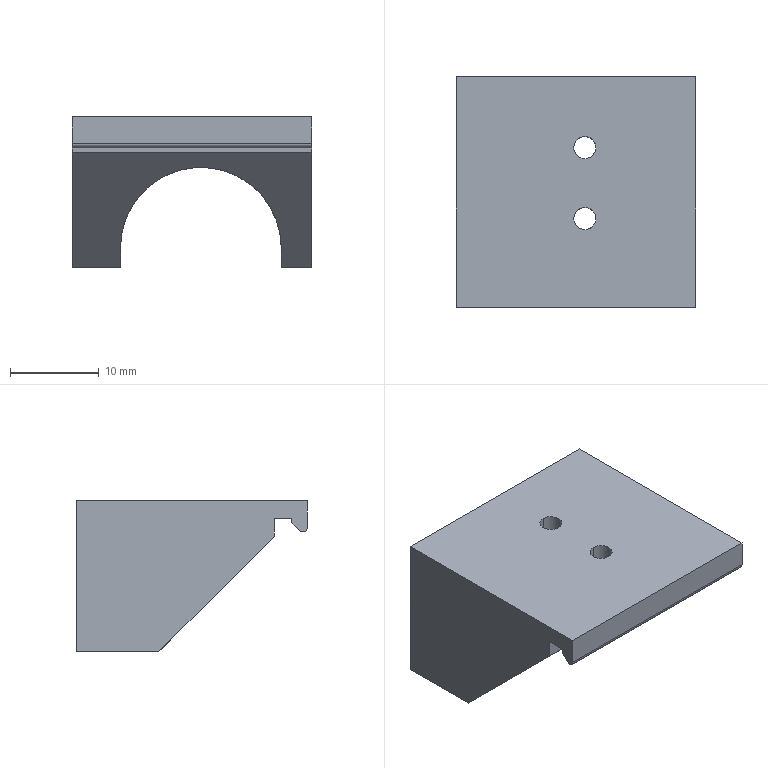Part | NX | 1 solid | 20 faces | box 27 x 26 x 17 mm | volume 5747 mm3 | plane 14 | cylinder 6 | commonest cylinder face diameters 2.5 x4 1 x1 18.14 x1
STEP:
#1=CARTESIAN_POINT('',(1.,-4.25,-5.73));
#2=VERTEX_POINT('',#1);
#3=CARTESIAN_POINT('',(1.,-1.75,-5.73));
#4=VERTEX_POINT('',#3);
#5=CARTESIAN_POINT('',(1.,-4.25,-5.73));
#6=CARTESIAN_POINT('',(1.331,-4.25,-5.73));
#7=CARTESIAN_POINT('',(1.978,-3.979,-5.773));
#8=CARTESIAN_POINT('',(2.386,-3.001,-5.838));
#9=CARTESIAN_POINT('',(1.978,-2.021,-5.773));
#10=CARTESIAN_POINT('',(1.331,-1.75,-5.73));
#11=CARTESIAN_POINT('',(1.,-1.75,-5.73));
#12=B_SPLINE_CURVE_WITH_KNOTS('',3,(#5,#6,#7,#8,#9,#10,#11),.UNSPECIFIED.,.F.,.F.,(4,1,1,1,4),(0.,0.000978,0.001956,0.002934,0.003912),.UNSPECIFIED.);
#13=EDGE_CURVE('',#2,#4,#12,.T.);
#14=ORIENTED_EDGE('',*,*,#13,.F.);
#15=CARTESIAN_POINT('',(1.,-4.25,0.));
#16=VERTEX_POINT('',#15);
#17=CARTESIAN_POINT('',(1.,-4.25,0.));
#18=DIRECTION('',(0.,0.,1.));
#19=VECTOR('',#18,1000.);
#20=LINE('',#17,#19);
#21=EDGE_CURVE('',#16,#2,#20,.F.);
#22=ORIENTED_EDGE('',*,*,#21,.F.);
#23=CARTESIAN_POINT('',(1.,-1.75,0.));
#24=VERTEX_POINT('',#23);
#25=CARTESIAN_POINT('',(1.,-3.,0.));
#26=DIRECTION('',(0.,0.,1.));
#27=DIRECTION('',(0.,1.,0.));
#28=AXIS2_PLACEMENT_3D('',#25,#26,#27);
#29=CIRCLE('',#28,1.25);
#30=EDGE_CURVE('',#16,#24,#29,.T.);
#31=ORIENTED_EDGE('',*,*,#30,.T.);
#32=CARTESIAN_POINT('',(1.,-1.75,0.));
#33=DIRECTION('',(0.,0.,1.));
#34=VECTOR('',#33,1000.);
#35=LINE('',#32,#34);
#36=EDGE_CURVE('',#24,#4,#35,.F.);
#37=ORIENTED_EDGE('',*,*,#36,.T.);
#38=EDGE_LOOP('',(#14,#22,#31,#37));
#39=FACE_BOUND('',#38,.T.);
#40=CARTESIAN_POINT('',(1.,-3.,0.));
#41=DIRECTION('',(0.,0.,1.));
#42=DIRECTION('',(0.,-1.,0.));
#43=AXIS2_PLACEMENT_3D('',#40,#41,#42);
#44=CYLINDRICAL_SURFACE('',#43,1.25);
#45=ADVANCED_FACE('',(#39),#44,.F.);
#46=CARTESIAN_POINT('',(1.,3.75,-5.73));
#47=VERTEX_POINT('',#46);
#48=CARTESIAN_POINT('',(1.,6.25,-5.73));
#49=VERTEX_POINT('',#48);
#50=CARTESIAN_POINT('',(1.,3.75,-5.73));
#51=CARTESIAN_POINT('',(1.331,3.75,-5.73));
#52=CARTESIAN_POINT('',(1.978,4.021,-5.773));
#53=CARTESIAN_POINT('',(2.386,4.999,-5.838));
#54=CARTESIAN_POINT('',(1.978,5.979,-5.773));
#55=CARTESIAN_POINT('',(1.331,6.25,-5.73));
#56=CARTESIAN_POINT('',(1.,6.25,-5.73));
#57=B_SPLINE_CURVE_WITH_KNOTS('',3,(#50,#51,#52,#53,#54,#55,#56),.UNSPECIFIED.,.F.,.F.,(4,1,1,1,4),(0.,0.000978,0.001956,0.002934,0.003912),.UNSPECIFIED.);
#58=EDGE_CURVE('',#47,#49,#57,.T.);
#59=ORIENTED_EDGE('',*,*,#58,.F.);
#60=CARTESIAN_POINT('',(1.,3.75,0.));
#61=VERTEX_POINT('',#60);
#62=CARTESIAN_POINT('',(1.,3.75,0.));
#63=DIRECTION('',(0.,0.,1.));
#64=VECTOR('',#63,1000.);
#65=LINE('',#62,#64);
#66=EDGE_CURVE('',#61,#47,#65,.F.);
#67=ORIENTED_EDGE('',*,*,#66,.F.);
#68=CARTESIAN_POINT('',(1.,6.25,0.));
#69=VERTEX_POINT('',#68);
#70=CARTESIAN_POINT('',(1.,5.,0.));
#71=DIRECTION('',(0.,0.,1.));
#72=DIRECTION('',(0.,1.,0.));
#73=AXIS2_PLACEMENT_3D('',#70,#71,#72);
#74=CIRCLE('',#73,1.25);
#75=EDGE_CURVE('',#61,#69,#74,.T.);
#76=ORIENTED_EDGE('',*,*,#75,.T.);
#77=CARTESIAN_POINT('',(1.,6.25,0.));
#78=DIRECTION('',(0.,0.,1.));
#79=VECTOR('',#78,1000.);
#80=LINE('',#77,#79);
#81=EDGE_CURVE('',#69,#49,#80,.F.);
#82=ORIENTED_EDGE('',*,*,#81,.T.);
#83=EDGE_LOOP('',(#59,#67,#76,#82));
#84=FACE_BOUND('',#83,.T.);
#85=CARTESIAN_POINT('',(1.,5.,0.));
#86=DIRECTION('',(0.,0.,1.));
#87=DIRECTION('',(0.,-1.,0.));
#88=AXIS2_PLACEMENT_3D('',#85,#86,#87);
#89=CYLINDRICAL_SURFACE('',#88,1.25);
#90=ADVANCED_FACE('',(#84),#89,.F.);
#91=CARTESIAN_POINT('',(-8.07,3.73,-17.));
#92=VERTEX_POINT('',#91);
#93=CARTESIAN_POINT('',(-8.07,13.,-17.));
#94=VERTEX_POINT('',#93);
#95=CARTESIAN_POINT('',(-8.07,0.,-17.));
#96=DIRECTION('',(0.,1.,0.));
#97=VECTOR('',#96,1000.);
#98=LINE('',#95,#97);
#99=EDGE_CURVE('',#92,#94,#98,.T.);
#100=ORIENTED_EDGE('',*,*,#99,.F.);
#101=CARTESIAN_POINT('',(-13.5,3.73,-17.));
#102=VERTEX_POINT('',#101);
#103=CARTESIAN_POINT('',(13.5,3.73,-17.));
#104=DIRECTION('',(-1.,0.,0.));
#105=VECTOR('',#104,1000.);
#106=LINE('',#103,#105);
#107=EDGE_CURVE('',#92,#102,#106,.T.);
#108=ORIENTED_EDGE('',*,*,#107,.T.);
#109=CARTESIAN_POINT('',(-13.5,13.,-17.));
#110=VERTEX_POINT('',#109);
#111=CARTESIAN_POINT('',(-13.5,13.,-17.));
#112=DIRECTION('',(0.,1.,0.));
#113=VECTOR('',#112,1000.);
#114=LINE('',#111,#113);
#115=EDGE_CURVE('',#102,#110,#114,.T.);
#116=ORIENTED_EDGE('',*,*,#115,.T.);
#117=CARTESIAN_POINT('',(13.5,13.,-17.));
#118=DIRECTION('',(1.,0.,0.));
#119=VECTOR('',#118,1000.);
#120=LINE('',#117,#119);
#121=EDGE_CURVE('',#110,#94,#120,.T.);
#122=ORIENTED_EDGE('',*,*,#121,.T.);
#123=EDGE_LOOP('',(#100,#108,#116,#122));
#124=FACE_BOUND('',#123,.T.);
#125=CARTESIAN_POINT('',(0.,0.,-17.));
#126=DIRECTION('',(0.,0.,-1.));
#127=DIRECTION('',(0.,1.,0.));
#128=AXIS2_PLACEMENT_3D('',#125,#126,#127);
#129=PLANE('',#128);
#130=ADVANCED_FACE('',(#124),#129,.T.);
#131=CARTESIAN_POINT('',(-13.5,-12.146,-3.376));
#132=VERTEX_POINT('',#131);
#133=CARTESIAN_POINT('',(-13.5,-11.27,-2.5));
#134=VERTEX_POINT('',#133);
#135=CARTESIAN_POINT('',(-13.5,-11.02,-2.25));
#136=DIRECTION('',(0.,0.7071,0.7071));
#137=VECTOR('',#136,1000.);
#138=LINE('',#135,#137);
#139=EDGE_CURVE('',#132,#134,#138,.T.);
#140=ORIENTED_EDGE('',*,*,#139,.F.);
#141=CARTESIAN_POINT('',(-13.5,-13.,-3.023));
#142=VERTEX_POINT('',#141);
#143=CARTESIAN_POINT('',(-13.5,-12.5,-3.023));
#144=DIRECTION('',(-1.,0.,0.));
#145=DIRECTION('',(0.,-1.,0.));
#146=AXIS2_PLACEMENT_3D('',#143,#144,#145);
#147=CIRCLE('',#146,0.5);
#148=EDGE_CURVE('',#132,#142,#147,.T.);
#149=ORIENTED_EDGE('',*,*,#148,.T.);
#150=CARTESIAN_POINT('',(-13.5,-13.,0.));
#151=VERTEX_POINT('',#150);
#152=CARTESIAN_POINT('',(-13.5,-13.,-17.));
#153=DIRECTION('',(0.,0.,1.));
#154=VECTOR('',#153,1000.);
#155=LINE('',#152,#154);
#156=EDGE_CURVE('',#142,#151,#155,.T.);
#157=ORIENTED_EDGE('',*,*,#156,.T.);
#158=CARTESIAN_POINT('',(-13.5,13.,0.));
#159=VERTEX_POINT('',#158);
#160=CARTESIAN_POINT('',(-13.5,13.,0.));
#161=DIRECTION('',(0.,1.,0.));
#162=VECTOR('',#161,1000.);
#163=LINE('',#160,#162);
#164=EDGE_CURVE('',#151,#159,#163,.T.);
#165=ORIENTED_EDGE('',*,*,#164,.T.);
#166=CARTESIAN_POINT('',(-13.5,13.,-17.));
#167=DIRECTION('',(0.,0.,1.));
#168=VECTOR('',#167,1000.);
#169=LINE('',#166,#168);
#170=EDGE_CURVE('',#110,#159,#169,.T.);
#171=ORIENTED_EDGE('',*,*,#170,.F.);
#172=ORIENTED_EDGE('',*,*,#115,.F.);
#173=CARTESIAN_POINT('',(-13.5,-9.27,-4.));
#174=VERTEX_POINT('',#173);
#175=CARTESIAN_POINT('',(-13.5,-11.02,-2.25));
#176=DIRECTION('',(0.,0.7071,-0.7071));
#177=VECTOR('',#176,1000.);
#178=LINE('',#175,#177);
#179=EDGE_CURVE('',#174,#102,#178,.T.);
#180=ORIENTED_EDGE('',*,*,#179,.F.);
#181=CARTESIAN_POINT('',(-13.5,-9.27,-2.));
#182=VERTEX_POINT('',#181);
#183=CARTESIAN_POINT('',(-13.5,-9.27,-2.));
#184=DIRECTION('',(0.,0.,-1.));
#185=VECTOR('',#184,1000.);
#186=LINE('',#183,#185);
#187=EDGE_CURVE('',#182,#174,#186,.T.);
#188=ORIENTED_EDGE('',*,*,#187,.F.);
#189=CARTESIAN_POINT('',(-13.5,-11.27,-2.));
#190=VERTEX_POINT('',#189);
#191=CARTESIAN_POINT('',(-13.5,-11.27,-2.));
#192=DIRECTION('',(0.,1.,0.));
#193=VECTOR('',#192,1000.);
#194=LINE('',#191,#193);
#195=EDGE_CURVE('',#190,#182,#194,.T.);
#196=ORIENTED_EDGE('',*,*,#195,.F.);
#197=CARTESIAN_POINT('',(-13.5,-11.27,-2.5));
#198=DIRECTION('',(0.,0.,1.));
#199=VECTOR('',#198,1000.);
#200=LINE('',#197,#199);
#201=EDGE_CURVE('',#134,#190,#200,.T.);
#202=ORIENTED_EDGE('',*,*,#201,.F.);
#203=EDGE_LOOP('',(#140,#149,#157,#165,#171,#172,#180,#188,#196,#202));
#204=FACE_BOUND('',#203,.T.);
#205=CARTESIAN_POINT('',(-13.5,13.,-17.));
#206=DIRECTION('',(1.,0.,0.));
#207=DIRECTION('',(0.,1.,0.));
#208=AXIS2_PLACEMENT_3D('',#205,#206,#207);
#209=PLANE('',#208);
#210=ADVANCED_FACE('',(#204),#209,.F.);
#211=CARTESIAN_POINT('',(-8.07,13.,-14.8));
#212=VERTEX_POINT('',#211);
#213=CARTESIAN_POINT('',(10.07,13.,-14.8));
#214=VERTEX_POINT('',#213);
#215=CARTESIAN_POINT('',(1.,13.,-14.8));
#216=DIRECTION('',(0.,-1.,0.));
#217=DIRECTION('',(0.,0.,-1.));
#218=AXIS2_PLACEMENT_3D('',#215,#216,#217);
#219=CIRCLE('',#218,9.07);
#220=EDGE_CURVE('',#212,#214,#219,.F.);
#221=ORIENTED_EDGE('',*,*,#220,.F.);
#222=CARTESIAN_POINT('',(-8.07,13.,-17.));
#223=DIRECTION('',(0.,0.,1.));
#224=VECTOR('',#223,1000.);
#225=LINE('',#222,#224);
#226=EDGE_CURVE('',#94,#212,#225,.T.);
#227=ORIENTED_EDGE('',*,*,#226,.F.);
#228=ORIENTED_EDGE('',*,*,#121,.F.);
#229=ORIENTED_EDGE('',*,*,#170,.T.);
#230=CARTESIAN_POINT('',(13.5,13.,0.));
#231=VERTEX_POINT('',#230);
#232=CARTESIAN_POINT('',(13.5,13.,0.));
#233=DIRECTION('',(1.,0.,0.));
#234=VECTOR('',#233,1000.);
#235=LINE('',#232,#234);
#236=EDGE_CURVE('',#159,#231,#235,.T.);
#237=ORIENTED_EDGE('',*,*,#236,.T.);
#238=CARTESIAN_POINT('',(13.5,13.,-17.));
#239=VERTEX_POINT('',#238);
#240=CARTESIAN_POINT('',(13.5,13.,-17.));
#241=DIRECTION('',(0.,0.,1.));
#242=VECTOR('',#241,1000.);
#243=LINE('',#240,#242);
#244=EDGE_CURVE('',#239,#231,#243,.T.);
#245=ORIENTED_EDGE('',*,*,#244,.F.);
#246=CARTESIAN_POINT('',(10.07,13.,-17.));
#247=VERTEX_POINT('',#246);
#248=CARTESIAN_POINT('',(13.5,13.,-17.));
#249=DIRECTION('',(1.,0.,0.));
#250=VECTOR('',#249,1000.);
#251=LINE('',#248,#250);
#252=EDGE_CURVE('',#247,#239,#251,.T.);
#253=ORIENTED_EDGE('',*,*,#252,.F.);
#254=CARTESIAN_POINT('',(10.07,13.,-17.));
#255=DIRECTION('',(0.,0.,-1.));
#256=VECTOR('',#255,1000.);
#257=LINE('',#254,#256);
#258=EDGE_CURVE('',#214,#247,#257,.T.);
#259=ORIENTED_EDGE('',*,*,#258,.F.);
#260=EDGE_LOOP('',(#221,#227,#228,#229,#237,#245,#253,#259));
#261=FACE_BOUND('',#260,.T.);
#262=CARTESIAN_POINT('',(13.5,13.,-17.));
#263=DIRECTION('',(0.,-1.,0.));
#264=DIRECTION('',(1.,0.,0.));
#265=AXIS2_PLACEMENT_3D('',#262,#263,#264);
#266=PLANE('',#265);
#267=ADVANCED_FACE('',(#261),#266,.F.);
#268=CARTESIAN_POINT('',(13.5,-13.,-3.023));
#269=VERTEX_POINT('',#268);
#270=CARTESIAN_POINT('',(13.5,-13.,0.));
#271=VERTEX_POINT('',#270);
#272=CARTESIAN_POINT('',(13.5,-13.,-17.));
#273=DIRECTION('',(0.,0.,1.));
#274=VECTOR('',#273,1000.);
#275=LINE('',#272,#274);
#276=EDGE_CURVE('',#269,#271,#275,.T.);
#277=ORIENTED_EDGE('',*,*,#276,.F.);
#278=CARTESIAN_POINT('',(13.5,-12.146,-3.376));
#279=VERTEX_POINT('',#278);
#280=CARTESIAN_POINT('',(13.5,-12.5,-3.023));
#281=DIRECTION('',(1.,0.,0.));
#282=DIRECTION('',(0.,1.,0.));
#283=AXIS2_PLACEMENT_3D('',#280,#281,#282);
#284=CIRCLE('',#283,0.5);
#285=EDGE_CURVE('',#269,#279,#284,.T.);
#286=ORIENTED_EDGE('',*,*,#285,.T.);
#287=CARTESIAN_POINT('',(13.5,-11.27,-2.5));
#288=VERTEX_POINT('',#287);
#289=CARTESIAN_POINT('',(13.5,-11.02,-2.25));
#290=DIRECTION('',(0.,0.7071,0.7071));
#291=VECTOR('',#290,1000.);
#292=LINE('',#289,#291);
#293=EDGE_CURVE('',#279,#288,#292,.T.);
#294=ORIENTED_EDGE('',*,*,#293,.T.);
#295=CARTESIAN_POINT('',(13.5,-11.27,-2.));
#296=VERTEX_POINT('',#295);
#297=CARTESIAN_POINT('',(13.5,-11.27,-2.5));
#298=DIRECTION('',(0.,0.,1.));
#299=VECTOR('',#298,1000.);
#300=LINE('',#297,#299);
#301=EDGE_CURVE('',#288,#296,#300,.T.);
#302=ORIENTED_EDGE('',*,*,#301,.T.);
#303=CARTESIAN_POINT('',(13.5,-9.27,-2.));
#304=VERTEX_POINT('',#303);
#305=CARTESIAN_POINT('',(13.5,-11.27,-2.));
#306=DIRECTION('',(0.,1.,0.));
#307=VECTOR('',#306,1000.);
#308=LINE('',#305,#307);
#309=EDGE_CURVE('',#296,#304,#308,.T.);
#310=ORIENTED_EDGE('',*,*,#309,.T.);
#311=CARTESIAN_POINT('',(13.5,-9.27,-4.));
#312=VERTEX_POINT('',#311);
#313=CARTESIAN_POINT('',(13.5,-9.27,-17.));
#314=DIRECTION('',(0.,0.,-1.));
#315=VECTOR('',#314,1000.);
#316=LINE('',#313,#315);
#317=EDGE_CURVE('',#304,#312,#316,.T.);
#318=ORIENTED_EDGE('',*,*,#317,.T.);
#319=CARTESIAN_POINT('',(13.5,3.73,-17.));
#320=VERTEX_POINT('',#319);
#321=CARTESIAN_POINT('',(13.5,-11.02,-2.25));
#322=DIRECTION('',(0.,0.7071,-0.7071));
#323=VECTOR('',#322,1000.);
#324=LINE('',#321,#323);
#325=EDGE_CURVE('',#312,#320,#324,.T.);
#326=ORIENTED_EDGE('',*,*,#325,.T.);
#327=CARTESIAN_POINT('',(13.5,13.,-17.));
#328=DIRECTION('',(0.,-1.,0.));
#329=VECTOR('',#328,1000.);
#330=LINE('',#327,#329);
#331=EDGE_CURVE('',#239,#320,#330,.T.);
#332=ORIENTED_EDGE('',*,*,#331,.F.);
#333=ORIENTED_EDGE('',*,*,#244,.T.);
#334=CARTESIAN_POINT('',(13.5,13.,0.));
#335=DIRECTION('',(0.,-1.,0.));
#336=VECTOR('',#335,1000.);
#337=LINE('',#334,#336);
#338=EDGE_CURVE('',#231,#271,#337,.T.);
#339=ORIENTED_EDGE('',*,*,#338,.T.);
#340=EDGE_LOOP('',(#277,#286,#294,#302,#310,#318,#326,#332,#333,#339));
#341=FACE_BOUND('',#340,.T.);
#342=CARTESIAN_POINT('',(13.5,13.,-17.));
#343=DIRECTION('',(-1.,0.,0.));
#344=DIRECTION('',(0.,-1.,0.));
#345=AXIS2_PLACEMENT_3D('',#342,#343,#344);
#346=PLANE('',#345);
#347=ADVANCED_FACE('',(#341),#346,.F.);
#348=ORIENTED_EDGE('',*,*,#156,.F.);
#349=CARTESIAN_POINT('',(13.5,-13.,-3.023));
#350=DIRECTION('',(1.,0.,0.));
#351=VECTOR('',#350,1000.);
#352=LINE('',#349,#351);
#353=EDGE_CURVE('',#142,#269,#352,.T.);
#354=ORIENTED_EDGE('',*,*,#353,.T.);
#355=ORIENTED_EDGE('',*,*,#276,.T.);
#356=CARTESIAN_POINT('',(13.5,-13.,0.));
#357=DIRECTION('',(-1.,0.,0.));
#358=VECTOR('',#357,1000.);
#359=LINE('',#356,#358);
#360=EDGE_CURVE('',#271,#151,#359,.T.);
#361=ORIENTED_EDGE('',*,*,#360,.T.);
#362=EDGE_LOOP('',(#348,#354,#355,#361));
#363=FACE_BOUND('',#362,.T.);
#364=CARTESIAN_POINT('',(13.5,-13.,-17.));
#365=DIRECTION('',(0.,1.,0.));
#366=DIRECTION('',(-1.,0.,0.));
#367=AXIS2_PLACEMENT_3D('',#364,#365,#366);
#368=PLANE('',#367);
#369=ADVANCED_FACE('',(#363),#368,.F.);
#370=CARTESIAN_POINT('',(10.07,3.73,-17.));
#371=VERTEX_POINT('',#370);
#372=CARTESIAN_POINT('',(10.07,-13.,-17.));
#373=DIRECTION('',(0.,1.,0.));
#374=VECTOR('',#373,1000.);
#375=LINE('',#372,#374);
#376=EDGE_CURVE('',#371,#247,#375,.T.);
#377=ORIENTED_EDGE('',*,*,#376,.T.);
#378=ORIENTED_EDGE('',*,*,#252,.T.);
#379=ORIENTED_EDGE('',*,*,#331,.T.);
#380=CARTESIAN_POINT('',(13.5,3.73,-17.));
#381=DIRECTION('',(-1.,0.,0.));
#382=VECTOR('',#381,1000.);
#383=LINE('',#380,#382);
#384=EDGE_CURVE('',#320,#371,#383,.T.);
#385=ORIENTED_EDGE('',*,*,#384,.T.);
#386=EDGE_LOOP('',(#377,#378,#379,#385));
#387=FACE_BOUND('',#386,.T.);
#388=CARTESIAN_POINT('',(0.,0.,-17.));
#389=DIRECTION('',(0.,0.,-1.));
#390=DIRECTION('',(0.,1.,0.));
#391=AXIS2_PLACEMENT_3D('',#388,#389,#390);
#392=PLANE('',#391);
#393=ADVANCED_FACE('',(#387),#392,.T.);
#394=CARTESIAN_POINT('',(1.,-3.,0.));
#395=DIRECTION('',(0.,0.,1.));
#396=DIRECTION('',(0.,1.,0.));
#397=AXIS2_PLACEMENT_3D('',#394,#395,#396);
#398=CIRCLE('',#397,1.25);
#399=EDGE_CURVE('',#24,#16,#398,.T.);
#400=ORIENTED_EDGE('',*,*,#399,.F.);
#401=ORIENTED_EDGE('',*,*,#30,.F.);
#402=EDGE_LOOP('',(#400,#401));
#403=FACE_BOUND('',#402,.T.);
#404=CARTESIAN_POINT('',(1.,5.,0.));
#405=DIRECTION('',(0.,0.,1.));
#406=DIRECTION('',(0.,1.,0.));
#407=AXIS2_PLACEMENT_3D('',#404,#405,#406);
#408=CIRCLE('',#407,1.25);
#409=EDGE_CURVE('',#69,#61,#408,.T.);
#410=ORIENTED_EDGE('',*,*,#409,.F.);
#411=ORIENTED_EDGE('',*,*,#75,.F.);
#412=EDGE_LOOP('',(#410,#411));
#413=FACE_BOUND('',#412,.T.);
#414=ORIENTED_EDGE('',*,*,#164,.F.);
#415=ORIENTED_EDGE('',*,*,#360,.F.);
#416=ORIENTED_EDGE('',*,*,#338,.F.);
#417=ORIENTED_EDGE('',*,*,#236,.F.);
#418=EDGE_LOOP('',(#414,#415,#416,#417));
#419=FACE_BOUND('',#418,.T.);
#420=CARTESIAN_POINT('',(0.,0.,0.));
#421=DIRECTION('',(0.,0.,-1.));
#422=DIRECTION('',(0.,1.,0.));
#423=AXIS2_PLACEMENT_3D('',#420,#421,#422);
#424=PLANE('',#423);
#425=ADVANCED_FACE('',(#403,#413,#419),#424,.F.);
#426=ORIENTED_EDGE('',*,*,#107,.F.);
#427=CARTESIAN_POINT('',(-8.07,1.53,-14.8));
#428=VERTEX_POINT('',#427);
#429=CARTESIAN_POINT('',(-8.07,-11.02,-2.25));
#430=DIRECTION('',(0.,-0.7071,0.7071));
#431=VECTOR('',#430,1000.);
#432=LINE('',#429,#431);
#433=EDGE_CURVE('',#92,#428,#432,.T.);
#434=ORIENTED_EDGE('',*,*,#433,.T.);
#435=CARTESIAN_POINT('',(10.07,1.53,-14.8));
#436=VERTEX_POINT('',#435);
#437=CARTESIAN_POINT('',(1.,1.53,-14.8));
#438=DIRECTION('',(0.,0.7071,0.7071));
#439=DIRECTION('',(0.,0.7071,-0.7071));
#440=AXIS2_PLACEMENT_3D('',#437,#438,#439);
#441=ELLIPSE('',#440,12.827,9.07);
#442=EDGE_CURVE('',#428,#436,#441,.T.);
#443=ORIENTED_EDGE('',*,*,#442,.T.);
#444=CARTESIAN_POINT('',(10.07,-11.02,-2.25));
#445=DIRECTION('',(0.,0.7071,-0.7071));
#446=VECTOR('',#445,1000.);
#447=LINE('',#444,#446);
#448=EDGE_CURVE('',#436,#371,#447,.T.);
#449=ORIENTED_EDGE('',*,*,#448,.T.);
#450=ORIENTED_EDGE('',*,*,#384,.F.);
#451=ORIENTED_EDGE('',*,*,#325,.F.);
#452=CARTESIAN_POINT('',(13.5,-9.27,-4.));
#453=DIRECTION('',(-1.,0.,0.));
#454=VECTOR('',#453,1000.);
#455=LINE('',#452,#454);
#456=EDGE_CURVE('',#312,#174,#455,.T.);
#457=ORIENTED_EDGE('',*,*,#456,.T.);
#458=ORIENTED_EDGE('',*,*,#179,.T.);
#459=EDGE_LOOP('',(#426,#434,#443,#449,#450,#451,#457,#458));
#460=FACE_BOUND('',#459,.T.);
#461=CARTESIAN_POINT('',(13.5,-11.02,-2.25));
#462=DIRECTION('',(0.,0.7071,0.7071));
#463=DIRECTION('',(0.,-0.7071,0.7071));
#464=AXIS2_PLACEMENT_3D('',#461,#462,#463);
#465=PLANE('',#464);
#466=ADVANCED_FACE('',(#460),#465,.F.);
#467=ORIENTED_EDGE('',*,*,#293,.F.);
#468=CARTESIAN_POINT('',(13.5,-12.146,-3.376));
#469=DIRECTION('',(-1.,0.,0.));
#470=VECTOR('',#469,1000.);
#471=LINE('',#468,#470);
#472=EDGE_CURVE('',#279,#132,#471,.T.);
#473=ORIENTED_EDGE('',*,*,#472,.T.);
#474=ORIENTED_EDGE('',*,*,#139,.T.);
#475=CARTESIAN_POINT('',(13.5,-11.27,-2.5));
#476=DIRECTION('',(-1.,0.,0.));
#477=VECTOR('',#476,1000.);
#478=LINE('',#475,#477);
#479=EDGE_CURVE('',#288,#134,#478,.T.);
#480=ORIENTED_EDGE('',*,*,#479,.F.);
#481=EDGE_LOOP('',(#467,#473,#474,#480));
#482=FACE_BOUND('',#481,.T.);
#483=CARTESIAN_POINT('',(13.5,-11.02,-2.25));
#484=DIRECTION('',(0.,-0.7071,0.7071));
#485=DIRECTION('',(0.,-0.7071,-0.7071));
#486=AXIS2_PLACEMENT_3D('',#483,#484,#485);
#487=PLANE('',#486);
#488=ADVANCED_FACE('',(#482),#487,.F.);
#489=ORIENTED_EDGE('',*,*,#187,.T.);
#490=ORIENTED_EDGE('',*,*,#456,.F.);
#491=ORIENTED_EDGE('',*,*,#317,.F.);
#492=CARTESIAN_POINT('',(13.5,-9.27,-2.));
#493=DIRECTION('',(-1.,0.,0.));
#494=VECTOR('',#493,1000.);
#495=LINE('',#492,#494);
#496=EDGE_CURVE('',#304,#182,#495,.T.);
#497=ORIENTED_EDGE('',*,*,#496,.T.);
#498=EDGE_LOOP('',(#489,#490,#491,#497));
#499=FACE_BOUND('',#498,.T.);
#500=CARTESIAN_POINT('',(13.5,-9.27,-2.));
#501=DIRECTION('',(0.,1.,0.));
#502=DIRECTION('',(-1.,0.,0.));
#503=AXIS2_PLACEMENT_3D('',#500,#501,#502);
#504=PLANE('',#503);
#505=ADVANCED_FACE('',(#499),#504,.F.);
#506=ORIENTED_EDGE('',*,*,#195,.T.);
#507=ORIENTED_EDGE('',*,*,#496,.F.);
#508=ORIENTED_EDGE('',*,*,#309,.F.);
#509=CARTESIAN_POINT('',(13.5,-11.27,-2.));
#510=DIRECTION('',(-1.,0.,0.));
#511=VECTOR('',#510,1000.);
#512=LINE('',#509,#511);
#513=EDGE_CURVE('',#296,#190,#512,.T.);
#514=ORIENTED_EDGE('',*,*,#513,.T.);
#515=EDGE_LOOP('',(#506,#507,#508,#514));
#516=FACE_BOUND('',#515,.T.);
#517=CARTESIAN_POINT('',(13.5,-11.27,-2.));
#518=DIRECTION('',(0.,0.,1.));
#519=DIRECTION('',(0.,-1.,0.));
#520=AXIS2_PLACEMENT_3D('',#517,#518,#519);
#521=PLANE('',#520);
#522=ADVANCED_FACE('',(#516),#521,.F.);
#523=ORIENTED_EDGE('',*,*,#201,.T.);
#524=ORIENTED_EDGE('',*,*,#513,.F.);
#525=ORIENTED_EDGE('',*,*,#301,.F.);
#526=ORIENTED_EDGE('',*,*,#479,.T.);
#527=EDGE_LOOP('',(#523,#524,#525,#526));
#528=FACE_BOUND('',#527,.T.);
#529=CARTESIAN_POINT('',(13.5,-11.27,-2.5));
#530=DIRECTION('',(0.,-1.,0.));
#531=DIRECTION('',(1.,0.,0.));
#532=AXIS2_PLACEMENT_3D('',#529,#530,#531);
#533=PLANE('',#532);
#534=ADVANCED_FACE('',(#528),#533,.F.);
#535=ORIENTED_EDGE('',*,*,#285,.F.);
#536=ORIENTED_EDGE('',*,*,#353,.F.);
#537=ORIENTED_EDGE('',*,*,#148,.F.);
#538=ORIENTED_EDGE('',*,*,#472,.F.);
#539=EDGE_LOOP('',(#535,#536,#537,#538));
#540=FACE_BOUND('',#539,.T.);
#541=CARTESIAN_POINT('',(13.5,-12.5,-3.023));
#542=DIRECTION('',(-1.,0.,0.));
#543=DIRECTION('',(0.,-1.,0.));
#544=AXIS2_PLACEMENT_3D('',#541,#542,#543);
#545=CYLINDRICAL_SURFACE('',#544,0.5);
#546=ADVANCED_FACE('',(#540),#545,.T.);
#547=CARTESIAN_POINT('',(1.,-1.75,-5.73));
#548=CARTESIAN_POINT('',(0.6695,-1.75,-5.73));
#549=CARTESIAN_POINT('',(0.02191,-2.021,-5.773));
#550=CARTESIAN_POINT('',(-0.3856,-2.999,-5.838));
#551=CARTESIAN_POINT('',(0.02049,-3.98,-5.773));
#552=CARTESIAN_POINT('',(0.6735,-4.25,-5.73));
#553=CARTESIAN_POINT('',(1.,-4.25,-5.73));
#554=B_SPLINE_CURVE_WITH_KNOTS('',3,(#547,#548,#549,#550,#551,#552,#553),.UNSPECIFIED.,.F.,.F.,(4,1,1,1,4),(0.0008326,0.001811,0.002789,0.003767,0.004745),.UNSPECIFIED.);
#555=EDGE_CURVE('',#4,#2,#554,.T.);
#556=ORIENTED_EDGE('',*,*,#555,.T.);
#557=ORIENTED_EDGE('',*,*,#13,.T.);
#558=EDGE_LOOP('',(#556,#557));
#559=FACE_BOUND('',#558,.T.);
#560=CARTESIAN_POINT('',(1.,6.25,-5.73));
#561=CARTESIAN_POINT('',(0.6695,6.25,-5.73));
#562=CARTESIAN_POINT('',(0.02191,5.979,-5.773));
#563=CARTESIAN_POINT('',(-0.3856,5.001,-5.838));
#564=CARTESIAN_POINT('',(0.02049,4.02,-5.773));
#565=CARTESIAN_POINT('',(0.6735,3.75,-5.73));
#566=CARTESIAN_POINT('',(1.,3.75,-5.73));
#567=B_SPLINE_CURVE_WITH_KNOTS('',3,(#560,#561,#562,#563,#564,#565,#566),.UNSPECIFIED.,.F.,.F.,(4,1,1,1,4),(0.0008326,0.001811,0.002789,0.003767,0.004745),.UNSPECIFIED.);
#568=EDGE_CURVE('',#49,#47,#567,.T.);
#569=ORIENTED_EDGE('',*,*,#568,.T.);
#570=ORIENTED_EDGE('',*,*,#58,.T.);
#571=EDGE_LOOP('',(#569,#570));
#572=FACE_BOUND('',#571,.T.);
#573=CARTESIAN_POINT('',(-8.07,-13.,-14.8));
#574=DIRECTION('',(0.,1.,0.));
#575=VECTOR('',#574,1000.);
#576=LINE('',#573,#575);
#577=EDGE_CURVE('',#428,#212,#576,.T.);
#578=ORIENTED_EDGE('',*,*,#577,.T.);
#579=ORIENTED_EDGE('',*,*,#220,.T.);
#580=CARTESIAN_POINT('',(10.07,-13.,-14.8));
#581=DIRECTION('',(0.,1.,0.));
#582=VECTOR('',#581,1000.);
#583=LINE('',#580,#582);
#584=EDGE_CURVE('',#436,#214,#583,.T.);
#585=ORIENTED_EDGE('',*,*,#584,.F.);
#586=ORIENTED_EDGE('',*,*,#442,.F.);
#587=EDGE_LOOP('',(#578,#579,#585,#586));
#588=FACE_BOUND('',#587,.T.);
#589=CARTESIAN_POINT('',(1.,-13.,-14.8));
#590=DIRECTION('',(0.,1.,0.));
#591=DIRECTION('',(-1.,0.,0.));
#592=AXIS2_PLACEMENT_3D('',#589,#590,#591);
#593=CYLINDRICAL_SURFACE('',#592,9.07);
#594=ADVANCED_FACE('',(#559,#572,#588),#593,.F.);
#595=ORIENTED_EDGE('',*,*,#99,.T.);
#596=ORIENTED_EDGE('',*,*,#226,.T.);
#597=ORIENTED_EDGE('',*,*,#577,.F.);
#598=ORIENTED_EDGE('',*,*,#433,.F.);
#599=EDGE_LOOP('',(#595,#596,#597,#598));
#600=FACE_BOUND('',#599,.T.);
#601=CARTESIAN_POINT('',(-8.07,-13.,-17.));
#602=DIRECTION('',(-1.,0.,0.));
#603=DIRECTION('',(0.,0.,1.));
#604=AXIS2_PLACEMENT_3D('',#601,#602,#603);
#605=PLANE('',#604);
#606=ADVANCED_FACE('',(#600),#605,.F.);
#607=ORIENTED_EDGE('',*,*,#584,.T.);
#608=ORIENTED_EDGE('',*,*,#258,.T.);
#609=ORIENTED_EDGE('',*,*,#376,.F.);
#610=ORIENTED_EDGE('',*,*,#448,.F.);
#611=EDGE_LOOP('',(#607,#608,#609,#610));
#612=FACE_BOUND('',#611,.T.);
#613=CARTESIAN_POINT('',(10.07,-13.,-17.));
#614=DIRECTION('',(1.,0.,0.));
#615=DIRECTION('',(0.,1.,0.));
#616=AXIS2_PLACEMENT_3D('',#613,#614,#615);
#617=PLANE('',#616);
#618=ADVANCED_FACE('',(#612),#617,.F.);
#619=ORIENTED_EDGE('',*,*,#66,.T.);
#620=ORIENTED_EDGE('',*,*,#568,.F.);
#621=ORIENTED_EDGE('',*,*,#81,.F.);
#622=ORIENTED_EDGE('',*,*,#409,.T.);
#623=EDGE_LOOP('',(#619,#620,#621,#622));
#624=FACE_BOUND('',#623,.T.);
#625=CARTESIAN_POINT('',(1.,5.,0.));
#626=DIRECTION('',(0.,0.,1.));
#627=DIRECTION('',(0.,-1.,0.));
#628=AXIS2_PLACEMENT_3D('',#625,#626,#627);
#629=CYLINDRICAL_SURFACE('',#628,1.25);
#630=ADVANCED_FACE('',(#624),#629,.F.);
#631=ORIENTED_EDGE('',*,*,#21,.T.);
#632=ORIENTED_EDGE('',*,*,#555,.F.);
#633=ORIENTED_EDGE('',*,*,#36,.F.);
#634=ORIENTED_EDGE('',*,*,#399,.T.);
#635=EDGE_LOOP('',(#631,#632,#633,#634));
#636=FACE_BOUND('',#635,.T.);
#637=CARTESIAN_POINT('',(1.,-3.,0.));
#638=DIRECTION('',(0.,0.,1.));
#639=DIRECTION('',(0.,-1.,0.));
#640=AXIS2_PLACEMENT_3D('',#637,#638,#639);
#641=CYLINDRICAL_SURFACE('',#640,1.25);
#642=ADVANCED_FACE('',(#636),#641,.F.);
#643=CLOSED_SHELL('',(#45,#90,#130,#210,#267,#347,#369,#393,#425,#466,#488,#505,#522,#534,#546,#594,#606,#618,#630,#642));
#644=MANIFOLD_SOLID_BREP('',#643);
#645=(LENGTH_UNIT()NAMED_UNIT(*)SI_UNIT(.MILLI.,.METRE.));
#646=UNCERTAINTY_MEASURE_WITH_UNIT(LENGTH_MEASURE(0.0508),#645,'','');
#647=(NAMED_UNIT(*)PLANE_ANGLE_UNIT()SI_UNIT($,.RADIAN.));
#648=(NAMED_UNIT(*)SI_UNIT($,.STERADIAN.)SOLID_ANGLE_UNIT());
#649=(GEOMETRIC_REPRESENTATION_CONTEXT(3)GLOBAL_UNCERTAINTY_ASSIGNED_CONTEXT((#646))GLOBAL_UNIT_ASSIGNED_CONTEXT((#645,#647,#648))REPRESENTATION_CONTEXT('',''));
#650=ADVANCED_BREP_SHAPE_REPRESENTATION('',(#644),#649);